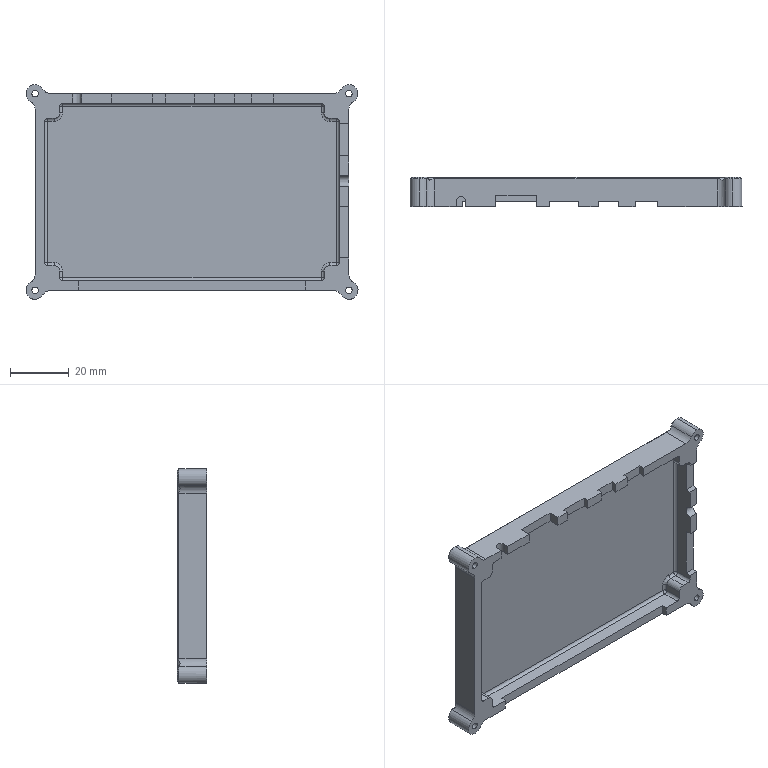Part | SolidWorks | features BaseBody 1 | 1 solid | 138 faces | box 113.2 x 10 x 73.2 mm | volume 29648 mm3 | plane 58 | cylinder 56 | cone 12 | spline 12 | commonest cylinder face diameters 2 x20 2.2 x8 6 x8 4 x6 6.2 x6 3.8 x4